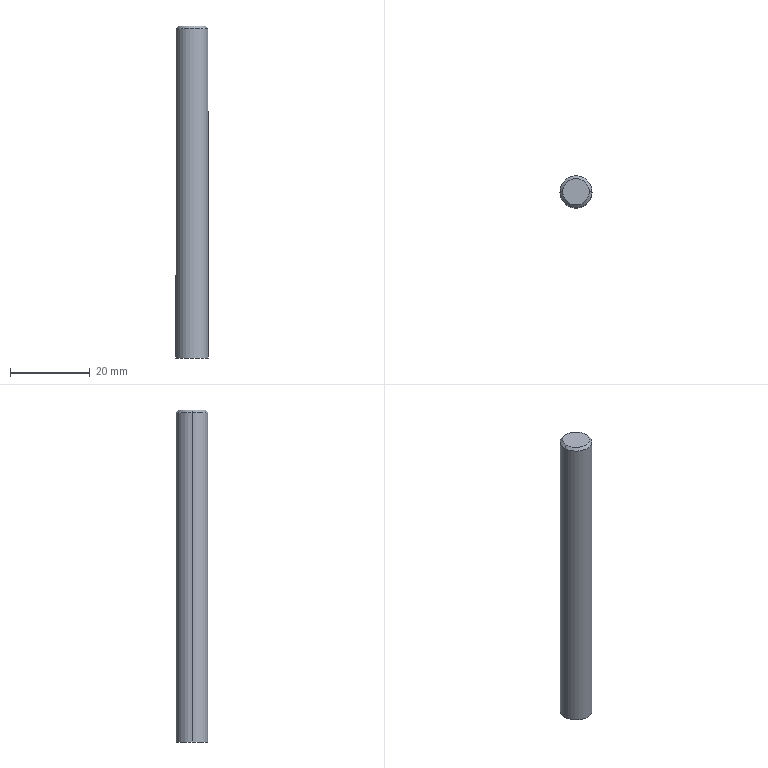Part | SolidWorks | features Extrusion 1, StudWizard 1 | 1 solid | 6 faces | box 8 x 8 x 83 mm | volume 4167 mm3 | cone 2 | cylinder 2 | plane 2 | commonest cylinder face diameters 8 x2
STEP:
#1=CARTESIAN_POINT('',(-73.324,-100.,64.));
#2=VERTEX_POINT('',#1);
#3=CARTESIAN_POINT('',(-66.677,-100.,64.));
#4=VERTEX_POINT('',#3);
#5=CARTESIAN_POINT('',(-70.,-100.,64.));
#6=DIRECTION('',(0.,0.,-1.));
#7=DIRECTION('',(-1.,0.,0.));
#8=AXIS2_PLACEMENT_3D('',#5,#6,#7);
#9=CIRCLE('',#8,3.323);
#10=EDGE_CURVE('',#2,#4,#9,.T.);
#11=ORIENTED_EDGE('',*,*,#10,.T.);
#12=CARTESIAN_POINT('',(-66.,-100.,63.324));
#13=VERTEX_POINT('',#12);
#14=CARTESIAN_POINT('',(-66.677,-100.,64.));
#15=DIRECTION('',(0.7071,0.,-0.7071));
#16=VECTOR('',#15,1000.);
#17=LINE('',#14,#16);
#18=EDGE_CURVE('',#4,#13,#17,.T.);
#19=ORIENTED_EDGE('',*,*,#18,.T.);
#20=CARTESIAN_POINT('',(-74.,-100.,63.324));
#21=VERTEX_POINT('',#20);
#22=CARTESIAN_POINT('',(-70.,-100.,63.324));
#23=DIRECTION('',(0.,0.,-1.));
#24=DIRECTION('',(-1.,0.,0.));
#25=AXIS2_PLACEMENT_3D('',#22,#23,#24);
#26=CIRCLE('',#25,4.);
#27=EDGE_CURVE('',#21,#13,#26,.T.);
#28=ORIENTED_EDGE('',*,*,#27,.F.);
#29=CARTESIAN_POINT('',(-73.324,-100.,64.));
#30=DIRECTION('',(-0.7071,0.,-0.7071));
#31=VECTOR('',#30,1000.);
#32=LINE('',#29,#31);
#33=EDGE_CURVE('',#2,#21,#32,.T.);
#34=ORIENTED_EDGE('',*,*,#33,.F.);
#35=EDGE_LOOP('',(#11,#19,#28,#34));
#36=FACE_OUTER_BOUND('',#35,.T.);
#37=CARTESIAN_POINT('',(-70.,-100.,64.));
#38=DIRECTION('',(0.,0.,-1.));
#39=DIRECTION('',(-1.,0.,0.));
#40=AXIS2_PLACEMENT_3D('',#37,#38,#39);
#41=CONICAL_SURFACE('',#40,3.323,0.7854);
#42=ADVANCED_FACE('',(#36),#41,.T.);
#43=ORIENTED_EDGE('',*,*,#27,.T.);
#44=CARTESIAN_POINT('',(-66.,-100.,-19.));
#45=VERTEX_POINT('',#44);
#46=CARTESIAN_POINT('',(-66.,-100.,64.));
#47=DIRECTION('',(0.,0.,-1.));
#48=VECTOR('',#47,1000.);
#49=LINE('',#46,#48);
#50=EDGE_CURVE('',#13,#45,#49,.T.);
#51=ORIENTED_EDGE('',*,*,#50,.T.);
#52=CARTESIAN_POINT('',(-74.,-100.,-19.));
#53=VERTEX_POINT('',#52);
#54=CARTESIAN_POINT('',(-70.,-100.,-19.));
#55=DIRECTION('',(0.,0.,-1.));
#56=DIRECTION('',(-1.,0.,0.));
#57=AXIS2_PLACEMENT_3D('',#54,#55,#56);
#58=CIRCLE('',#57,4.);
#59=EDGE_CURVE('',#53,#45,#58,.T.);
#60=ORIENTED_EDGE('',*,*,#59,.F.);
#61=CARTESIAN_POINT('',(-74.,-100.,64.));
#62=DIRECTION('',(0.,0.,-1.));
#63=VECTOR('',#62,1000.);
#64=LINE('',#61,#63);
#65=EDGE_CURVE('',#21,#53,#64,.T.);
#66=ORIENTED_EDGE('',*,*,#65,.F.);
#67=EDGE_LOOP('',(#43,#51,#60,#66));
#68=FACE_OUTER_BOUND('',#67,.T.);
#69=CARTESIAN_POINT('',(-70.,-100.,64.));
#70=DIRECTION('',(0.,0.,-1.));
#71=DIRECTION('',(-1.,0.,0.));
#72=AXIS2_PLACEMENT_3D('',#69,#70,#71);
#73=CYLINDRICAL_SURFACE('',#72,4.);
#74=ADVANCED_FACE('',(#68),#73,.T.);
#75=ORIENTED_EDGE('',*,*,#10,.F.);
#76=CARTESIAN_POINT('',(-70.,-100.,64.));
#77=DIRECTION('',(0.,0.,-1.));
#78=DIRECTION('',(-1.,0.,0.));
#79=AXIS2_PLACEMENT_3D('',#76,#77,#78);
#80=CIRCLE('',#79,3.323);
#81=EDGE_CURVE('',#4,#2,#80,.T.);
#82=ORIENTED_EDGE('',*,*,#81,.F.);
#83=EDGE_LOOP('',(#75,#82));
#84=FACE_OUTER_BOUND('',#83,.T.);
#85=CARTESIAN_POINT('',(-70.,-100.,64.));
#86=DIRECTION('',(0.,0.,1.));
#87=DIRECTION('',(1.,0.,0.));
#88=AXIS2_PLACEMENT_3D('',#85,#86,#87);
#89=PLANE('',#88);
#90=ADVANCED_FACE('',(#84),#89,.T.);
#91=ORIENTED_EDGE('',*,*,#50,.F.);
#92=CARTESIAN_POINT('',(-70.,-100.,63.324));
#93=DIRECTION('',(0.,0.,-1.));
#94=DIRECTION('',(-1.,0.,0.));
#95=AXIS2_PLACEMENT_3D('',#92,#93,#94);
#96=CIRCLE('',#95,4.);
#97=EDGE_CURVE('',#13,#21,#96,.T.);
#98=ORIENTED_EDGE('',*,*,#97,.T.);
#99=ORIENTED_EDGE('',*,*,#65,.T.);
#100=CARTESIAN_POINT('',(-70.,-100.,-19.));
#101=DIRECTION('',(0.,0.,-1.));
#102=DIRECTION('',(-1.,0.,0.));
#103=AXIS2_PLACEMENT_3D('',#100,#101,#102);
#104=CIRCLE('',#103,4.);
#105=EDGE_CURVE('',#45,#53,#104,.T.);
#106=ORIENTED_EDGE('',*,*,#105,.F.);
#107=EDGE_LOOP('',(#91,#98,#99,#106));
#108=FACE_OUTER_BOUND('',#107,.T.);
#109=CARTESIAN_POINT('',(-70.,-100.,64.));
#110=DIRECTION('',(0.,0.,-1.));
#111=DIRECTION('',(-1.,0.,0.));
#112=AXIS2_PLACEMENT_3D('',#109,#110,#111);
#113=CYLINDRICAL_SURFACE('',#112,4.);
#114=ADVANCED_FACE('',(#108),#113,.T.);
#115=ORIENTED_EDGE('',*,*,#18,.F.);
#116=ORIENTED_EDGE('',*,*,#81,.T.);
#117=ORIENTED_EDGE('',*,*,#33,.T.);
#118=ORIENTED_EDGE('',*,*,#97,.F.);
#119=EDGE_LOOP('',(#115,#116,#117,#118));
#120=FACE_OUTER_BOUND('',#119,.T.);
#121=CARTESIAN_POINT('',(-70.,-100.,64.));
#122=DIRECTION('',(0.,0.,-1.));
#123=DIRECTION('',(-1.,0.,0.));
#124=AXIS2_PLACEMENT_3D('',#121,#122,#123);
#125=CONICAL_SURFACE('',#124,3.323,0.7854);
#126=ADVANCED_FACE('',(#120),#125,.T.);
#127=ORIENTED_EDGE('',*,*,#59,.T.);
#128=ORIENTED_EDGE('',*,*,#105,.T.);
#129=EDGE_LOOP('',(#127,#128));
#130=FACE_OUTER_BOUND('',#129,.T.);
#131=CARTESIAN_POINT('',(-70.,-100.,-19.));
#132=DIRECTION('',(0.,0.,1.));
#133=DIRECTION('',(1.,0.,0.));
#134=AXIS2_PLACEMENT_3D('',#131,#132,#133);
#135=PLANE('',#134);
#136=ADVANCED_FACE('',(#130),#135,.F.);
#137=CLOSED_SHELL('',(#42,#74,#90,#114,#126,#136));
#138=MANIFOLD_SOLID_BREP('',#137);
#139=CARTESIAN_POINT('',(0.,0.,0.));
#140=DIRECTION('',(0.,0.,1.));
#141=DIRECTION('',(1.,0.,0.));
#142=AXIS2_PLACEMENT_3D('',#139,#140,#141);
#143=(LENGTH_UNIT()NAMED_UNIT(*)SI_UNIT(.MILLI.,.METRE.));
#144=UNCERTAINTY_MEASURE_WITH_UNIT(LENGTH_MEASURE(0.00001),#143,'','');
#145=(NAMED_UNIT(*)PLANE_ANGLE_UNIT()SI_UNIT($,.RADIAN.));
#146=(NAMED_UNIT(*)SI_UNIT($,.STERADIAN.)SOLID_ANGLE_UNIT());
#147=(GEOMETRIC_REPRESENTATION_CONTEXT(3)GLOBAL_UNCERTAINTY_ASSIGNED_CONTEXT((#144))GLOBAL_UNIT_ASSIGNED_CONTEXT((#143,#145,#146))REPRESENTATION_CONTEXT('',''));
#148=ADVANCED_BREP_SHAPE_REPRESENTATION('',(#138,#142),#147);